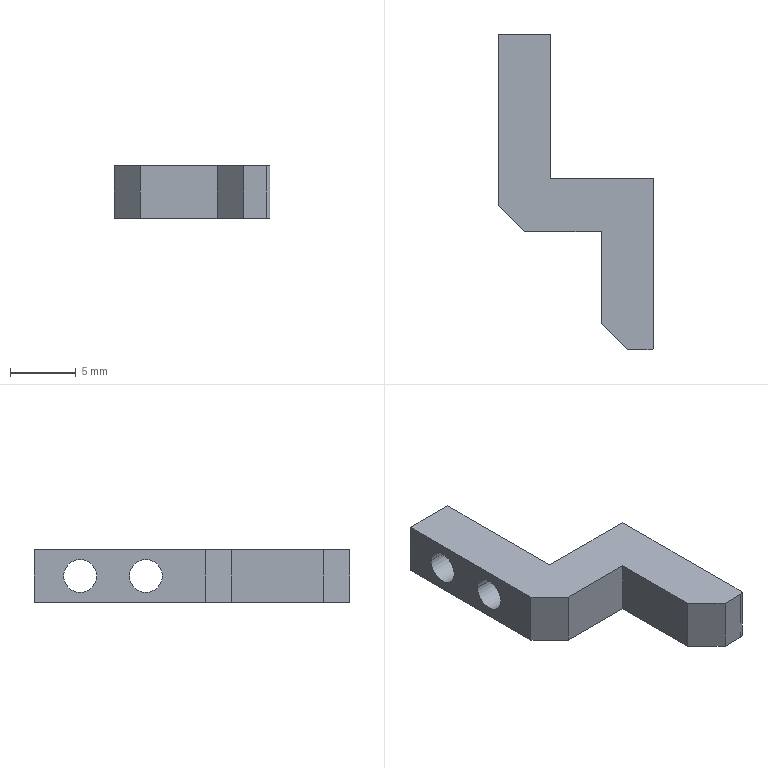Part | STEP file | Gripper_Default | 1 solid | 17 faces | box 11.85 x 24 x 4 mm | volume 454.253 mm3 | plane 12 | cylinder 5 | commonest cylinder face diameters 2.5 x4 0.6 x1
STEP:
#1=CARTESIAN_POINT('',(0.,0.,0.));
#2=DIRECTION('',(0.,0.,1.));
#3=DIRECTION('',(1.,0.,0.));
#4=AXIS2_PLACEMENT_3D('',#1,#2,#3);
#5=CARTESIAN_POINT('',(0.,-2.25,2.));
#6=VERTEX_POINT('',#5);
#7=CARTESIAN_POINT('',(4.,-2.25,2.));
#8=VERTEX_POINT('',#7);
#9=CARTESIAN_POINT('',(0.,-2.25,2.));
#10=DIRECTION('',(1.,0.,0.));
#11=VECTOR('',#10,1.);
#12=LINE('',#9,#11);
#13=CARTESIAN_POINT('',(0.,-3.5,2.));
#14=DIRECTION('',(1.,0.,0.));
#15=DIRECTION('',(0.,1.,0.));
#16=AXIS2_PLACEMENT_3D('',#13,#14,#15);
#17=CYLINDRICAL_SURFACE('',#16,1.25);
#18=CARTESIAN_POINT('',(6.283,0.));
#19=DIRECTION('',(0.,1.));
#20=VECTOR('',#19,1.);
#21=LINE('',#18,#20);
#22=(GEOMETRIC_REPRESENTATION_CONTEXT(2)PARAMETRIC_REPRESENTATION_CONTEXT()REPRESENTATION_CONTEXT('',''));
#23=DEFINITIONAL_REPRESENTATION('',(#21),#22);
#24=PCURVE('',#17,#23);
#25=CARTESIAN_POINT('',(0.,-3.5,2.));
#26=DIRECTION('',(1.,0.,0.));
#27=DIRECTION('',(0.,1.,0.));
#28=AXIS2_PLACEMENT_3D('',#25,#26,#27);
#29=CYLINDRICAL_SURFACE('',#28,1.25);
#30=CARTESIAN_POINT('',(0.,0.));
#31=DIRECTION('',(0.,1.));
#32=VECTOR('',#31,1.);
#33=LINE('',#30,#32);
#34=(GEOMETRIC_REPRESENTATION_CONTEXT(2)PARAMETRIC_REPRESENTATION_CONTEXT()REPRESENTATION_CONTEXT('',''));
#35=DEFINITIONAL_REPRESENTATION('',(#33),#34);
#36=PCURVE('',#29,#35);
#37=SURFACE_CURVE('',#12,(#24,#36),.PCURVE_S1.);
#38=EDGE_CURVE('',#6,#8,#37,.T.);
#39=ORIENTED_EDGE('',*,*,#38,.T.);
#40=CARTESIAN_POINT('',(4.,-4.75,2.));
#41=VERTEX_POINT('',#40);
#42=CARTESIAN_POINT('',(4.,-3.5,2.));
#43=DIRECTION('',(1.,0.,0.));
#44=DIRECTION('',(0.,1.,0.));
#45=AXIS2_PLACEMENT_3D('',#42,#43,#44);
#46=CIRCLE('',#45,1.25);
#47=CARTESIAN_POINT('',(0.,4.));
#48=DIRECTION('',(1.,0.));
#49=VECTOR('',#48,1.);
#50=LINE('',#47,#49);
#51=(GEOMETRIC_REPRESENTATION_CONTEXT(2)PARAMETRIC_REPRESENTATION_CONTEXT()REPRESENTATION_CONTEXT('',''));
#52=DEFINITIONAL_REPRESENTATION('',(#50),#51);
#53=PCURVE('',#17,#52);
#54=CARTESIAN_POINT('',(4.,0.,4.));
#55=DIRECTION('',(-1.,0.,0.));
#56=DIRECTION('',(0.,-1.,0.));
#57=AXIS2_PLACEMENT_3D('',#54,#55,#56);
#58=PLANE('',#57);
#59=CARTESIAN_POINT('',(2.25,-2.));
#60=CARTESIAN_POINT('',(2.25,0.1651));
#61=CARTESIAN_POINT('',(4.125,-0.9175));
#62=CARTESIAN_POINT('',(6.,-2.));
#63=CARTESIAN_POINT('',(4.125,-3.083));
#64=CARTESIAN_POINT('',(2.25,-4.165));
#65=CARTESIAN_POINT('',(2.25,-2.));
#66=(BOUNDED_CURVE()B_SPLINE_CURVE(2,(#59,#60,#61,#62,#63,#64,#65),.UNSPECIFIED.,.T.,.F.)B_SPLINE_CURVE_WITH_KNOTS((1,2,2,2,2,1),(-2.094,0.,2.094,4.189,6.283,8.378),.UNSPECIFIED.)CURVE()GEOMETRIC_REPRESENTATION_ITEM()RATIONAL_B_SPLINE_CURVE((1.,0.5,1.,0.5,1.,0.5,1.))REPRESENTATION_ITEM(''));
#67=(GEOMETRIC_REPRESENTATION_CONTEXT(2)PARAMETRIC_REPRESENTATION_CONTEXT()REPRESENTATION_CONTEXT('',''));
#68=DEFINITIONAL_REPRESENTATION('',(#66),#67);
#69=PCURVE('',#58,#68);
#70=SURFACE_CURVE('',#46,(#53,#69),.PCURVE_S1.);
#71=EDGE_CURVE('',#41,#8,#70,.T.);
#72=ORIENTED_EDGE('',*,*,#71,.F.);
#73=CARTESIAN_POINT('',(0.,-4.75,2.));
#74=VERTEX_POINT('',#73);
#75=CARTESIAN_POINT('',(0.,-4.75,2.));
#76=DIRECTION('',(1.,0.,0.));
#77=VECTOR('',#76,1.);
#78=LINE('',#75,#77);
#79=CARTESIAN_POINT('',(3.142,0.));
#80=DIRECTION('',(0.,1.));
#81=VECTOR('',#80,1.);
#82=LINE('',#79,#81);
#83=(GEOMETRIC_REPRESENTATION_CONTEXT(2)PARAMETRIC_REPRESENTATION_CONTEXT()REPRESENTATION_CONTEXT('',''));
#84=DEFINITIONAL_REPRESENTATION('',(#82),#83);
#85=PCURVE('',#17,#84);
#86=CARTESIAN_POINT('',(3.142,0.));
#87=DIRECTION('',(0.,1.));
#88=VECTOR('',#87,1.);
#89=LINE('',#86,#88);
#90=(GEOMETRIC_REPRESENTATION_CONTEXT(2)PARAMETRIC_REPRESENTATION_CONTEXT()REPRESENTATION_CONTEXT('',''));
#91=DEFINITIONAL_REPRESENTATION('',(#89),#90);
#92=PCURVE('',#29,#91);
#93=SURFACE_CURVE('',#78,(#85,#92),.PCURVE_S1.);
#94=EDGE_CURVE('',#74,#41,#93,.T.);
#95=ORIENTED_EDGE('',*,*,#94,.F.);
#96=CARTESIAN_POINT('',(0.,-3.5,2.));
#97=DIRECTION('',(1.,0.,0.));
#98=DIRECTION('',(0.,1.,0.));
#99=AXIS2_PLACEMENT_3D('',#96,#97,#98);
#100=CIRCLE('',#99,1.25);
#101=CARTESIAN_POINT('',(0.,0.));
#102=DIRECTION('',(1.,0.));
#103=VECTOR('',#102,1.);
#104=LINE('',#101,#103);
#105=(GEOMETRIC_REPRESENTATION_CONTEXT(2)PARAMETRIC_REPRESENTATION_CONTEXT()REPRESENTATION_CONTEXT('',''));
#106=DEFINITIONAL_REPRESENTATION('',(#104),#105);
#107=PCURVE('',#17,#106);
#108=CARTESIAN_POINT('',(0.,0.,4.));
#109=DIRECTION('',(1.,0.,0.));
#110=DIRECTION('',(0.,1.,0.));
#111=AXIS2_PLACEMENT_3D('',#108,#109,#110);
#112=PLANE('',#111);
#113=CARTESIAN_POINT('',(-3.5,-2.));
#114=DIRECTION('',(1.,0.));
#115=AXIS2_PLACEMENT_2D('',#113,#114);
#116=CIRCLE('',#115,1.25);
#117=(GEOMETRIC_REPRESENTATION_CONTEXT(2)PARAMETRIC_REPRESENTATION_CONTEXT()REPRESENTATION_CONTEXT('',''));
#118=DEFINITIONAL_REPRESENTATION('',(#116),#117);
#119=PCURVE('',#112,#118);
#120=SURFACE_CURVE('',#100,(#107,#119),.PCURVE_S1.);
#121=EDGE_CURVE('',#74,#6,#120,.T.);
#122=ORIENTED_EDGE('',*,*,#121,.T.);
#123=EDGE_LOOP('',(#39,#72,#95,#122));
#124=FACE_BOUND('',#123,.F.);
#125=ADVANCED_FACE('',(#124),#17,.F.);
#126=CARTESIAN_POINT('',(0.,-7.25,2.));
#127=VERTEX_POINT('',#126);
#128=CARTESIAN_POINT('',(4.,-7.25,2.));
#129=VERTEX_POINT('',#128);
#130=CARTESIAN_POINT('',(0.,-7.25,2.));
#131=DIRECTION('',(1.,0.,0.));
#132=VECTOR('',#131,1.);
#133=LINE('',#130,#132);
#134=CARTESIAN_POINT('',(0.,-8.5,2.));
#135=DIRECTION('',(1.,0.,0.));
#136=DIRECTION('',(0.,1.,0.));
#137=AXIS2_PLACEMENT_3D('',#134,#135,#136);
#138=CYLINDRICAL_SURFACE('',#137,1.25);
#139=CARTESIAN_POINT('',(6.283,0.));
#140=DIRECTION('',(0.,1.));
#141=VECTOR('',#140,1.);
#142=LINE('',#139,#141);
#143=(GEOMETRIC_REPRESENTATION_CONTEXT(2)PARAMETRIC_REPRESENTATION_CONTEXT()REPRESENTATION_CONTEXT('',''));
#144=DEFINITIONAL_REPRESENTATION('',(#142),#143);
#145=PCURVE('',#138,#144);
#146=CARTESIAN_POINT('',(0.,-8.5,2.));
#147=DIRECTION('',(1.,0.,0.));
#148=DIRECTION('',(0.,1.,0.));
#149=AXIS2_PLACEMENT_3D('',#146,#147,#148);
#150=CYLINDRICAL_SURFACE('',#149,1.25);
#151=CARTESIAN_POINT('',(0.,0.));
#152=DIRECTION('',(0.,1.));
#153=VECTOR('',#152,1.);
#154=LINE('',#151,#153);
#155=(GEOMETRIC_REPRESENTATION_CONTEXT(2)PARAMETRIC_REPRESENTATION_CONTEXT()REPRESENTATION_CONTEXT('',''));
#156=DEFINITIONAL_REPRESENTATION('',(#154),#155);
#157=PCURVE('',#150,#156);
#158=SURFACE_CURVE('',#133,(#145,#157),.PCURVE_S1.);
#159=EDGE_CURVE('',#127,#129,#158,.T.);
#160=ORIENTED_EDGE('',*,*,#159,.T.);
#161=CARTESIAN_POINT('',(4.,-9.75,2.));
#162=VERTEX_POINT('',#161);
#163=CARTESIAN_POINT('',(4.,-8.5,2.));
#164=DIRECTION('',(1.,0.,0.));
#165=DIRECTION('',(0.,1.,0.));
#166=AXIS2_PLACEMENT_3D('',#163,#164,#165);
#167=CIRCLE('',#166,1.25);
#168=CARTESIAN_POINT('',(0.,4.));
#169=DIRECTION('',(1.,0.));
#170=VECTOR('',#169,1.);
#171=LINE('',#168,#170);
#172=(GEOMETRIC_REPRESENTATION_CONTEXT(2)PARAMETRIC_REPRESENTATION_CONTEXT()REPRESENTATION_CONTEXT('',''));
#173=DEFINITIONAL_REPRESENTATION('',(#171),#172);
#174=PCURVE('',#138,#173);
#175=CARTESIAN_POINT('',(7.25,-2.));
#176=CARTESIAN_POINT('',(7.25,0.1651));
#177=CARTESIAN_POINT('',(9.125,-0.9175));
#178=CARTESIAN_POINT('',(11.,-2.));
#179=CARTESIAN_POINT('',(9.125,-3.083));
#180=CARTESIAN_POINT('',(7.25,-4.165));
#181=CARTESIAN_POINT('',(7.25,-2.));
#182=(BOUNDED_CURVE()B_SPLINE_CURVE(2,(#175,#176,#177,#178,#179,#180,#181),.UNSPECIFIED.,.T.,.F.)B_SPLINE_CURVE_WITH_KNOTS((1,2,2,2,2,1),(-2.094,0.,2.094,4.189,6.283,8.378),.UNSPECIFIED.)CURVE()GEOMETRIC_REPRESENTATION_ITEM()RATIONAL_B_SPLINE_CURVE((1.,0.5,1.,0.5,1.,0.5,1.))REPRESENTATION_ITEM(''));
#183=(GEOMETRIC_REPRESENTATION_CONTEXT(2)PARAMETRIC_REPRESENTATION_CONTEXT()REPRESENTATION_CONTEXT('',''));
#184=DEFINITIONAL_REPRESENTATION('',(#182),#183);
#185=PCURVE('',#58,#184);
#186=SURFACE_CURVE('',#167,(#174,#185),.PCURVE_S1.);
#187=EDGE_CURVE('',#162,#129,#186,.T.);
#188=ORIENTED_EDGE('',*,*,#187,.F.);
#189=CARTESIAN_POINT('',(0.,-9.75,2.));
#190=VERTEX_POINT('',#189);
#191=CARTESIAN_POINT('',(0.,-9.75,2.));
#192=DIRECTION('',(1.,0.,0.));
#193=VECTOR('',#192,1.);
#194=LINE('',#191,#193);
#195=CARTESIAN_POINT('',(3.142,0.));
#196=DIRECTION('',(0.,1.));
#197=VECTOR('',#196,1.);
#198=LINE('',#195,#197);
#199=(GEOMETRIC_REPRESENTATION_CONTEXT(2)PARAMETRIC_REPRESENTATION_CONTEXT()REPRESENTATION_CONTEXT('',''));
#200=DEFINITIONAL_REPRESENTATION('',(#198),#199);
#201=PCURVE('',#138,#200);
#202=CARTESIAN_POINT('',(3.142,0.));
#203=DIRECTION('',(0.,1.));
#204=VECTOR('',#203,1.);
#205=LINE('',#202,#204);
#206=(GEOMETRIC_REPRESENTATION_CONTEXT(2)PARAMETRIC_REPRESENTATION_CONTEXT()REPRESENTATION_CONTEXT('',''));
#207=DEFINITIONAL_REPRESENTATION('',(#205),#206);
#208=PCURVE('',#150,#207);
#209=SURFACE_CURVE('',#194,(#201,#208),.PCURVE_S1.);
#210=EDGE_CURVE('',#190,#162,#209,.T.);
#211=ORIENTED_EDGE('',*,*,#210,.F.);
#212=CARTESIAN_POINT('',(0.,-8.5,2.));
#213=DIRECTION('',(1.,0.,0.));
#214=DIRECTION('',(0.,1.,0.));
#215=AXIS2_PLACEMENT_3D('',#212,#213,#214);
#216=CIRCLE('',#215,1.25);
#217=CARTESIAN_POINT('',(0.,0.));
#218=DIRECTION('',(1.,0.));
#219=VECTOR('',#218,1.);
#220=LINE('',#217,#219);
#221=(GEOMETRIC_REPRESENTATION_CONTEXT(2)PARAMETRIC_REPRESENTATION_CONTEXT()REPRESENTATION_CONTEXT('',''));
#222=DEFINITIONAL_REPRESENTATION('',(#220),#221);
#223=PCURVE('',#138,#222);
#224=CARTESIAN_POINT('',(-8.5,-2.));
#225=DIRECTION('',(1.,0.));
#226=AXIS2_PLACEMENT_2D('',#224,#225);
#227=CIRCLE('',#226,1.25);
#228=(GEOMETRIC_REPRESENTATION_CONTEXT(2)PARAMETRIC_REPRESENTATION_CONTEXT()REPRESENTATION_CONTEXT('',''));
#229=DEFINITIONAL_REPRESENTATION('',(#227),#228);
#230=PCURVE('',#112,#229);
#231=SURFACE_CURVE('',#216,(#223,#230),.PCURVE_S1.);
#232=EDGE_CURVE('',#190,#127,#231,.T.);
#233=ORIENTED_EDGE('',*,*,#232,.T.);
#234=EDGE_LOOP('',(#160,#188,#211,#233));
#235=FACE_BOUND('',#234,.F.);
#236=ADVANCED_FACE('',(#235),#138,.F.);
#237=CARTESIAN_POINT('',(0.,-3.5,2.));
#238=DIRECTION('',(1.,0.,0.));
#239=DIRECTION('',(0.,1.,0.));
#240=AXIS2_PLACEMENT_3D('',#237,#238,#239);
#241=CIRCLE('',#240,1.25);
#242=CARTESIAN_POINT('',(-3.5,-2.));
#243=DIRECTION('',(1.,0.));
#244=AXIS2_PLACEMENT_2D('',#242,#243);
#245=CIRCLE('',#244,1.25);
#246=(GEOMETRIC_REPRESENTATION_CONTEXT(2)PARAMETRIC_REPRESENTATION_CONTEXT()REPRESENTATION_CONTEXT('',''));
#247=DEFINITIONAL_REPRESENTATION('',(#245),#246);
#248=PCURVE('',#112,#247);
#249=CARTESIAN_POINT('',(0.,0.));
#250=DIRECTION('',(1.,0.));
#251=VECTOR('',#250,1.);
#252=LINE('',#249,#251);
#253=(GEOMETRIC_REPRESENTATION_CONTEXT(2)PARAMETRIC_REPRESENTATION_CONTEXT()REPRESENTATION_CONTEXT('',''));
#254=DEFINITIONAL_REPRESENTATION('',(#252),#253);
#255=PCURVE('',#29,#254);
#256=SURFACE_CURVE('',#241,(#248,#255),.PCURVE_S1.);
#257=EDGE_CURVE('',#6,#74,#256,.T.);
#258=ORIENTED_EDGE('',*,*,#257,.T.);
#259=ORIENTED_EDGE('',*,*,#121,.T.);
#260=EDGE_LOOP('',(#258,#259));
#261=FACE_BOUND('',#260,.T.);
#262=CARTESIAN_POINT('',(0.,-8.5,2.));
#263=DIRECTION('',(1.,0.,0.));
#264=DIRECTION('',(0.,1.,0.));
#265=AXIS2_PLACEMENT_3D('',#262,#263,#264);
#266=CIRCLE('',#265,1.25);
#267=CARTESIAN_POINT('',(-8.5,-2.));
#268=DIRECTION('',(1.,0.));
#269=AXIS2_PLACEMENT_2D('',#267,#268);
#270=CIRCLE('',#269,1.25);
#271=(GEOMETRIC_REPRESENTATION_CONTEXT(2)PARAMETRIC_REPRESENTATION_CONTEXT()REPRESENTATION_CONTEXT('',''));
#272=DEFINITIONAL_REPRESENTATION('',(#270),#271);
#273=PCURVE('',#112,#272);
#274=CARTESIAN_POINT('',(0.,0.));
#275=DIRECTION('',(1.,0.));
#276=VECTOR('',#275,1.);
#277=LINE('',#274,#276);
#278=(GEOMETRIC_REPRESENTATION_CONTEXT(2)PARAMETRIC_REPRESENTATION_CONTEXT()REPRESENTATION_CONTEXT('',''));
#279=DEFINITIONAL_REPRESENTATION('',(#277),#278);
#280=PCURVE('',#150,#279);
#281=SURFACE_CURVE('',#266,(#273,#280),.PCURVE_S1.);
#282=EDGE_CURVE('',#127,#190,#281,.T.);
#283=ORIENTED_EDGE('',*,*,#282,.T.);
#284=ORIENTED_EDGE('',*,*,#232,.T.);
#285=EDGE_LOOP('',(#283,#284));
#286=FACE_BOUND('',#285,.T.);
#287=CARTESIAN_POINT('',(0.,0.,0.));
#288=VERTEX_POINT('',#287);
#289=CARTESIAN_POINT('',(0.,-13.,0.));
#290=VERTEX_POINT('',#289);
#291=CARTESIAN_POINT('',(0.,0.,0.));
#292=DIRECTION('',(0.,-1.,0.));
#293=VECTOR('',#292,1.);
#294=LINE('',#291,#293);
#295=CARTESIAN_POINT('',(0.,-4.));
#296=DIRECTION('',(-1.,0.));
#297=VECTOR('',#296,1.);
#298=LINE('',#295,#297);
#299=(GEOMETRIC_REPRESENTATION_CONTEXT(2)PARAMETRIC_REPRESENTATION_CONTEXT()REPRESENTATION_CONTEXT('',''));
#300=DEFINITIONAL_REPRESENTATION('',(#298),#299);
#301=PCURVE('',#112,#300);
#302=CARTESIAN_POINT('',(0.,-24.,0.));
#303=DIRECTION('',(0.,0.,-1.));
#304=DIRECTION('',(-1.,0.,0.));
#305=AXIS2_PLACEMENT_3D('',#302,#303,#304);
#306=PLANE('',#305);
#307=CARTESIAN_POINT('',(0.,24.));
#308=DIRECTION('',(0.,-1.));
#309=VECTOR('',#308,1.);
#310=LINE('',#307,#309);
#311=(GEOMETRIC_REPRESENTATION_CONTEXT(2)PARAMETRIC_REPRESENTATION_CONTEXT()REPRESENTATION_CONTEXT('',''));
#312=DEFINITIONAL_REPRESENTATION('',(#310),#311);
#313=PCURVE('',#306,#312);
#314=SURFACE_CURVE('',#294,(#301,#313),.PCURVE_S1.);
#315=EDGE_CURVE('',#288,#290,#314,.T.);
#316=ORIENTED_EDGE('',*,*,#315,.T.);
#317=CARTESIAN_POINT('',(0.,-13.,4.));
#318=VERTEX_POINT('',#317);
#319=CARTESIAN_POINT('',(0.,-13.,4.));
#320=DIRECTION('',(0.,0.,1.));
#321=VECTOR('',#320,1.);
#322=LINE('',#319,#321);
#323=CARTESIAN_POINT('',(-13.,0.));
#324=DIRECTION('',(0.,1.));
#325=VECTOR('',#324,1.);
#326=LINE('',#323,#325);
#327=(GEOMETRIC_REPRESENTATION_CONTEXT(2)PARAMETRIC_REPRESENTATION_CONTEXT()REPRESENTATION_CONTEXT('',''));
#328=DEFINITIONAL_REPRESENTATION('',(#326),#327);
#329=PCURVE('',#112,#328);
#330=CARTESIAN_POINT('',(0.,-13.,4.));
#331=DIRECTION('',(0.7071,0.7071,0.));
#332=DIRECTION('',(-0.7071,0.7071,0.));
#333=AXIS2_PLACEMENT_3D('',#330,#331,#332);
#334=PLANE('',#333);
#335=CARTESIAN_POINT('',(0.,0.));
#336=DIRECTION('',(0.,1.));
#337=VECTOR('',#336,1.);
#338=LINE('',#335,#337);
#339=(GEOMETRIC_REPRESENTATION_CONTEXT(2)PARAMETRIC_REPRESENTATION_CONTEXT()REPRESENTATION_CONTEXT('',''));
#340=DEFINITIONAL_REPRESENTATION('',(#338),#339);
#341=PCURVE('',#334,#340);
#342=SURFACE_CURVE('',#322,(#329,#341),.PCURVE_S1.);
#343=EDGE_CURVE('',#290,#318,#342,.T.);
#344=ORIENTED_EDGE('',*,*,#343,.T.);
#345=CARTESIAN_POINT('',(0.,0.,4.));
#346=VERTEX_POINT('',#345);
#347=CARTESIAN_POINT('',(0.,0.,4.));
#348=DIRECTION('',(0.,-1.,0.));
#349=VECTOR('',#348,1.);
#350=LINE('',#347,#349);
#351=CARTESIAN_POINT('',(0.,0.));
#352=DIRECTION('',(-1.,0.));
#353=VECTOR('',#352,1.);
#354=LINE('',#351,#353);
#355=(GEOMETRIC_REPRESENTATION_CONTEXT(2)PARAMETRIC_REPRESENTATION_CONTEXT()REPRESENTATION_CONTEXT('',''));
#356=DEFINITIONAL_REPRESENTATION('',(#354),#355);
#357=PCURVE('',#112,#356);
#358=CARTESIAN_POINT('',(0.,-24.,4.));
#359=DIRECTION('',(0.,0.,-1.));
#360=DIRECTION('',(-1.,0.,0.));
#361=AXIS2_PLACEMENT_3D('',#358,#359,#360);
#362=PLANE('',#361);
#363=CARTESIAN_POINT('',(0.,24.));
#364=DIRECTION('',(0.,-1.));
#365=VECTOR('',#364,1.);
#366=LINE('',#363,#365);
#367=(GEOMETRIC_REPRESENTATION_CONTEXT(2)PARAMETRIC_REPRESENTATION_CONTEXT()REPRESENTATION_CONTEXT('',''));
#368=DEFINITIONAL_REPRESENTATION('',(#366),#367);
#369=PCURVE('',#362,#368);
#370=SURFACE_CURVE('',#350,(#357,#369),.PCURVE_S1.);
#371=EDGE_CURVE('',#346,#318,#370,.T.);
#372=ORIENTED_EDGE('',*,*,#371,.F.);
#373=CARTESIAN_POINT('',(0.,0.,4.));
#374=DIRECTION('',(0.,0.,-1.));
#375=VECTOR('',#374,1.);
#376=LINE('',#373,#375);
#377=CARTESIAN_POINT('',(0.,0.));
#378=DIRECTION('',(0.,-1.));
#379=VECTOR('',#378,1.);
#380=LINE('',#377,#379);
#381=(GEOMETRIC_REPRESENTATION_CONTEXT(2)PARAMETRIC_REPRESENTATION_CONTEXT()REPRESENTATION_CONTEXT('',''));
#382=DEFINITIONAL_REPRESENTATION('',(#380),#381);
#383=PCURVE('',#112,#382);
#384=CARTESIAN_POINT('',(0.,0.,4.));
#385=DIRECTION('',(0.,-1.,0.));
#386=DIRECTION('',(0.,0.,-1.));
#387=AXIS2_PLACEMENT_3D('',#384,#385,#386);
#388=PLANE('',#387);
#389=CARTESIAN_POINT('',(0.,0.));
#390=DIRECTION('',(1.,0.));
#391=VECTOR('',#390,1.);
#392=LINE('',#389,#391);
#393=(GEOMETRIC_REPRESENTATION_CONTEXT(2)PARAMETRIC_REPRESENTATION_CONTEXT()REPRESENTATION_CONTEXT('',''));
#394=DEFINITIONAL_REPRESENTATION('',(#392),#393);
#395=PCURVE('',#388,#394);
#396=SURFACE_CURVE('',#376,(#383,#395),.PCURVE_S1.);
#397=EDGE_CURVE('',#346,#288,#396,.T.);
#398=ORIENTED_EDGE('',*,*,#397,.T.);
#399=EDGE_LOOP('',(#316,#344,#372,#398));
#400=FACE_BOUND('',#399,.T.);
#401=ADVANCED_FACE('',(#261,#286,#400),#112,.F.);
#402=CARTESIAN_POINT('',(9.85,-24.,0.));
#403=VERTEX_POINT('',#402);
#404=CARTESIAN_POINT('',(11.55,-24.,0.));
#405=VERTEX_POINT('',#404);
#406=CARTESIAN_POINT('',(11.85,-24.,0.));
#407=DIRECTION('',(1.,0.,0.));
#408=VECTOR('',#407,1.);
#409=LINE('',#406,#408);
#410=CARTESIAN_POINT('',(11.85,-24.,4.));
#411=DIRECTION('',(0.,1.,0.));
#412=DIRECTION('',(0.,0.,1.));
#413=AXIS2_PLACEMENT_3D('',#410,#411,#412);
#414=PLANE('',#413);
#415=CARTESIAN_POINT('',(-4.,0.));
#416=DIRECTION('',(0.,1.));
#417=VECTOR('',#416,1.);
#418=LINE('',#415,#417);
#419=(GEOMETRIC_REPRESENTATION_CONTEXT(2)PARAMETRIC_REPRESENTATION_CONTEXT()REPRESENTATION_CONTEXT('',''));
#420=DEFINITIONAL_REPRESENTATION('',(#418),#419);
#421=PCURVE('',#414,#420);
#422=CARTESIAN_POINT('',(-11.85,0.));
#423=DIRECTION('',(-1.,0.));
#424=VECTOR('',#423,1.);
#425=LINE('',#422,#424);
#426=(GEOMETRIC_REPRESENTATION_CONTEXT(2)PARAMETRIC_REPRESENTATION_CONTEXT()REPRESENTATION_CONTEXT('',''));
#427=DEFINITIONAL_REPRESENTATION('',(#425),#426);
#428=PCURVE('',#306,#427);
#429=SURFACE_CURVE('',#409,(#421,#428),.PCURVE_S1.);
#430=EDGE_CURVE('',#403,#405,#429,.T.);
#431=ORIENTED_EDGE('',*,*,#430,.T.);
#432=CARTESIAN_POINT('',(11.55,-24.,4.));
#433=VERTEX_POINT('',#432);
#434=CARTESIAN_POINT('',(11.55,-24.,4.));
#435=DIRECTION('',(0.,0.,1.));
#436=VECTOR('',#435,1.);
#437=LINE('',#434,#436);
#438=CARTESIAN_POINT('',(0.,-0.3));
#439=DIRECTION('',(1.,0.));
#440=VECTOR('',#439,1.);
#441=LINE('',#438,#440);
#442=(GEOMETRIC_REPRESENTATION_CONTEXT(2)PARAMETRIC_REPRESENTATION_CONTEXT()REPRESENTATION_CONTEXT('',''));
#443=DEFINITIONAL_REPRESENTATION('',(#441),#442);
#444=PCURVE('',#414,#443);
#445=CARTESIAN_POINT('',(11.55,-23.7,4.));
#446=DIRECTION('',(0.,0.,-1.));
#447=DIRECTION('',(-1.,0.,0.));
#448=AXIS2_PLACEMENT_3D('',#445,#446,#447);
#449=CYLINDRICAL_SURFACE('',#448,0.3);
#450=CARTESIAN_POINT('',(4.712,0.));
#451=DIRECTION('',(0.,-1.));
#452=VECTOR('',#451,1.);
#453=LINE('',#450,#452);
#454=(GEOMETRIC_REPRESENTATION_CONTEXT(2)PARAMETRIC_REPRESENTATION_CONTEXT()REPRESENTATION_CONTEXT('',''));
#455=DEFINITIONAL_REPRESENTATION('',(#453),#454);
#456=PCURVE('',#449,#455);
#457=SURFACE_CURVE('',#437,(#444,#456),.PCURVE_S1.);
#458=EDGE_CURVE('',#405,#433,#457,.T.);
#459=ORIENTED_EDGE('',*,*,#458,.T.);
#460=CARTESIAN_POINT('',(9.85,-24.,4.));
#461=VERTEX_POINT('',#460);
#462=CARTESIAN_POINT('',(11.85,-24.,4.));
#463=DIRECTION('',(1.,0.,0.));
#464=VECTOR('',#463,1.);
#465=LINE('',#462,#464);
#466=CARTESIAN_POINT('',(0.,0.));
#467=DIRECTION('',(0.,1.));
#468=VECTOR('',#467,1.);
#469=LINE('',#466,#468);
#470=(GEOMETRIC_REPRESENTATION_CONTEXT(2)PARAMETRIC_REPRESENTATION_CONTEXT()REPRESENTATION_CONTEXT('',''));
#471=DEFINITIONAL_REPRESENTATION('',(#469),#470);
#472=PCURVE('',#414,#471);
#473=CARTESIAN_POINT('',(-11.85,0.));
#474=DIRECTION('',(-1.,0.));
#475=VECTOR('',#474,1.);
#476=LINE('',#473,#475);
#477=(GEOMETRIC_REPRESENTATION_CONTEXT(2)PARAMETRIC_REPRESENTATION_CONTEXT()REPRESENTATION_CONTEXT('',''));
#478=DEFINITIONAL_REPRESENTATION('',(#476),#477);
#479=PCURVE('',#362,#478);
#480=SURFACE_CURVE('',#465,(#472,#479),.PCURVE_S1.);
#481=EDGE_CURVE('',#461,#433,#480,.T.);
#482=ORIENTED_EDGE('',*,*,#481,.F.);
#483=CARTESIAN_POINT('',(9.85,-24.,4.));
#484=DIRECTION('',(0.,0.,-1.));
#485=VECTOR('',#484,1.);
#486=LINE('',#483,#485);
#487=CARTESIAN_POINT('',(0.,-2.));
#488=DIRECTION('',(-1.,0.));
#489=VECTOR('',#488,1.);
#490=LINE('',#487,#489);
#491=(GEOMETRIC_REPRESENTATION_CONTEXT(2)PARAMETRIC_REPRESENTATION_CONTEXT()REPRESENTATION_CONTEXT('',''));
#492=DEFINITIONAL_REPRESENTATION('',(#490),#491);
#493=PCURVE('',#414,#492);
#494=CARTESIAN_POINT('',(9.85,-24.,4.));
#495=DIRECTION('',(0.7071,0.7071,0.));
#496=DIRECTION('',(-0.7071,0.7071,0.));
#497=AXIS2_PLACEMENT_3D('',#494,#495,#496);
#498=PLANE('',#497);
#499=CARTESIAN_POINT('',(0.,0.));
#500=DIRECTION('',(0.,-1.));
#501=VECTOR('',#500,1.);
#502=LINE('',#499,#501);
#503=(GEOMETRIC_REPRESENTATION_CONTEXT(2)PARAMETRIC_REPRESENTATION_CONTEXT()REPRESENTATION_CONTEXT('',''));
#504=DEFINITIONAL_REPRESENTATION('',(#502),#503);
#505=PCURVE('',#498,#504);
#506=SURFACE_CURVE('',#486,(#493,#505),.PCURVE_S1.);
#507=EDGE_CURVE('',#461,#403,#506,.T.);
#508=ORIENTED_EDGE('',*,*,#507,.T.);
#509=EDGE_LOOP('',(#431,#459,#482,#508));
#510=FACE_BOUND('',#509,.T.);
#511=ADVANCED_FACE('',(#510),#414,.F.);
#512=CARTESIAN_POINT('',(11.85,-23.7,4.));
#513=VERTEX_POINT('',#512);
#514=CARTESIAN_POINT('',(11.85,-11.,4.));
#515=VERTEX_POINT('',#514);
#516=CARTESIAN_POINT('',(11.85,-11.,4.));
#517=DIRECTION('',(0.,1.,0.));
#518=VECTOR('',#517,1.);
#519=LINE('',#516,#518);
#520=CARTESIAN_POINT('',(11.85,-11.,4.));
#521=DIRECTION('',(-1.,0.,0.));
#522=DIRECTION('',(0.,-1.,0.));
#523=AXIS2_PLACEMENT_3D('',#520,#521,#522);
#524=PLANE('',#523);
#525=CARTESIAN_POINT('',(0.,0.));
#526=DIRECTION('',(-1.,0.));
#527=VECTOR('',#526,1.);
#528=LINE('',#525,#527);
#529=(GEOMETRIC_REPRESENTATION_CONTEXT(2)PARAMETRIC_REPRESENTATION_CONTEXT()REPRESENTATION_CONTEXT('',''));
#530=DEFINITIONAL_REPRESENTATION('',(#528),#529);
#531=PCURVE('',#524,#530);
#532=CARTESIAN_POINT('',(-11.85,13.));
#533=DIRECTION('',(0.,1.));
#534=VECTOR('',#533,1.);
#535=LINE('',#532,#534);
#536=(GEOMETRIC_REPRESENTATION_CONTEXT(2)PARAMETRIC_REPRESENTATION_CONTEXT()REPRESENTATION_CONTEXT('',''));
#537=DEFINITIONAL_REPRESENTATION('',(#535),#536);
#538=PCURVE('',#362,#537);
#539=SURFACE_CURVE('',#519,(#531,#538),.PCURVE_S1.);
#540=EDGE_CURVE('',#513,#515,#539,.T.);
#541=ORIENTED_EDGE('',*,*,#540,.F.);
#542=CARTESIAN_POINT('',(11.85,-23.7,0.));
#543=VERTEX_POINT('',#542);
#544=CARTESIAN_POINT('',(11.85,-23.7,4.));
#545=DIRECTION('',(0.,0.,-1.));
#546=VECTOR('',#545,1.);
#547=LINE('',#544,#546);
#548=CARTESIAN_POINT('',(12.7,0.));
#549=DIRECTION('',(0.,-1.));
#550=VECTOR('',#549,1.);
#551=LINE('',#548,#550);
#552=(GEOMETRIC_REPRESENTATION_CONTEXT(2)PARAMETRIC_REPRESENTATION_CONTEXT()REPRESENTATION_CONTEXT('',''));
#553=DEFINITIONAL_REPRESENTATION('',(#551),#552);
#554=PCURVE('',#524,#553);
#555=CARTESIAN_POINT('',(3.142,0.));
#556=DIRECTION('',(0.,1.));
#557=VECTOR('',#556,1.);
#558=LINE('',#555,#557);
#559=(GEOMETRIC_REPRESENTATION_CONTEXT(2)PARAMETRIC_REPRESENTATION_CONTEXT()REPRESENTATION_CONTEXT('',''));
#560=DEFINITIONAL_REPRESENTATION('',(#558),#559);
#561=PCURVE('',#449,#560);
#562=SURFACE_CURVE('',#547,(#554,#561),.PCURVE_S1.);
#563=EDGE_CURVE('',#513,#543,#562,.T.);
#564=ORIENTED_EDGE('',*,*,#563,.T.);
#565=CARTESIAN_POINT('',(11.85,-11.,0.));
#566=VERTEX_POINT('',#565);
#567=CARTESIAN_POINT('',(11.85,-11.,0.));
#568=DIRECTION('',(0.,1.,0.));
#569=VECTOR('',#568,1.);
#570=LINE('',#567,#569);
#571=CARTESIAN_POINT('',(0.,-4.));
#572=DIRECTION('',(-1.,0.));
#573=VECTOR('',#572,1.);
#574=LINE('',#571,#573);
#575=(GEOMETRIC_REPRESENTATION_CONTEXT(2)PARAMETRIC_REPRESENTATION_CONTEXT()REPRESENTATION_CONTEXT('',''));
#576=DEFINITIONAL_REPRESENTATION('',(#574),#575);
#577=PCURVE('',#524,#576);
#578=CARTESIAN_POINT('',(-11.85,13.));
#579=DIRECTION('',(0.,1.));
#580=VECTOR('',#579,1.);
#581=LINE('',#578,#580);
#582=(GEOMETRIC_REPRESENTATION_CONTEXT(2)PARAMETRIC_REPRESENTATION_CONTEXT()REPRESENTATION_CONTEXT('',''));
#583=DEFINITIONAL_REPRESENTATION('',(#581),#582);
#584=PCURVE('',#306,#583);
#585=SURFACE_CURVE('',#570,(#577,#584),.PCURVE_S1.);
#586=EDGE_CURVE('',#543,#566,#585,.T.);
#587=ORIENTED_EDGE('',*,*,#586,.T.);
#588=CARTESIAN_POINT('',(11.85,-11.,4.));
#589=DIRECTION('',(0.,0.,-1.));
#590=VECTOR('',#589,1.);
#591=LINE('',#588,#590);
#592=CARTESIAN_POINT('',(0.,0.));
#593=DIRECTION('',(0.,-1.));
#594=VECTOR('',#593,1.);
#595=LINE('',#592,#594);
#596=(GEOMETRIC_REPRESENTATION_CONTEXT(2)PARAMETRIC_REPRESENTATION_CONTEXT()REPRESENTATION_CONTEXT('',''));
#597=DEFINITIONAL_REPRESENTATION('',(#595),#596);
#598=PCURVE('',#524,#597);
#599=CARTESIAN_POINT('',(4.,-11.,4.));
#600=DIRECTION('',(0.,-1.,0.));
#601=DIRECTION('',(0.,0.,-1.));
#602=AXIS2_PLACEMENT_3D('',#599,#600,#601);
#603=PLANE('',#602);
#604=CARTESIAN_POINT('',(0.,7.85));
#605=DIRECTION('',(1.,0.));
#606=VECTOR('',#605,1.);
#607=LINE('',#604,#606);
#608=(GEOMETRIC_REPRESENTATION_CONTEXT(2)PARAMETRIC_REPRESENTATION_CONTEXT()REPRESENTATION_CONTEXT('',''));
#609=DEFINITIONAL_REPRESENTATION('',(#607),#608);
#610=PCURVE('',#603,#609);
#611=SURFACE_CURVE('',#591,(#598,#610),.PCURVE_S1.);
#612=EDGE_CURVE('',#515,#566,#611,.T.);
#613=ORIENTED_EDGE('',*,*,#612,.F.);
#614=EDGE_LOOP('',(#541,#564,#587,#613));
#615=FACE_BOUND('',#614,.T.);
#616=ADVANCED_FACE('',(#615),#524,.F.);
#617=CARTESIAN_POINT('',(4.,-11.,0.));
#618=VERTEX_POINT('',#617);
#619=CARTESIAN_POINT('',(4.,-11.,0.));
#620=DIRECTION('',(-1.,0.,0.));
#621=VECTOR('',#620,1.);
#622=LINE('',#619,#621);
#623=CARTESIAN_POINT('',(4.,0.));
#624=DIRECTION('',(0.,-1.));
#625=VECTOR('',#624,1.);
#626=LINE('',#623,#625);
#627=(GEOMETRIC_REPRESENTATION_CONTEXT(2)PARAMETRIC_REPRESENTATION_CONTEXT()REPRESENTATION_CONTEXT('',''));
#628=DEFINITIONAL_REPRESENTATION('',(#626),#627);
#629=PCURVE('',#603,#628);
#630=CARTESIAN_POINT('',(-4.,13.));
#631=DIRECTION('',(1.,0.));
#632=VECTOR('',#631,1.);
#633=LINE('',#630,#632);
#634=(GEOMETRIC_REPRESENTATION_CONTEXT(2)PARAMETRIC_REPRESENTATION_CONTEXT()REPRESENTATION_CONTEXT('',''));
#635=DEFINITIONAL_REPRESENTATION('',(#633),#634);
#636=PCURVE('',#306,#635);
#637=SURFACE_CURVE('',#622,(#629,#636),.PCURVE_S1.);
#638=EDGE_CURVE('',#566,#618,#637,.T.);
#639=ORIENTED_EDGE('',*,*,#638,.T.);
#640=CARTESIAN_POINT('',(4.,-11.,4.));
#641=VERTEX_POINT('',#640);
#642=CARTESIAN_POINT('',(4.,-11.,4.));
#643=DIRECTION('',(0.,0.,-1.));
#644=VECTOR('',#643,1.);
#645=LINE('',#642,#644);
#646=CARTESIAN_POINT('',(0.,0.));
#647=DIRECTION('',(1.,0.));
#648=VECTOR('',#647,1.);
#649=LINE('',#646,#648);
#650=(GEOMETRIC_REPRESENTATION_CONTEXT(2)PARAMETRIC_REPRESENTATION_CONTEXT()REPRESENTATION_CONTEXT('',''));
#651=DEFINITIONAL_REPRESENTATION('',(#649),#650);
#652=PCURVE('',#603,#651);
#653=CARTESIAN_POINT('',(11.,0.));
#654=DIRECTION('',(0.,-1.));
#655=VECTOR('',#654,1.);
#656=LINE('',#653,#655);
#657=(GEOMETRIC_REPRESENTATION_CONTEXT(2)PARAMETRIC_REPRESENTATION_CONTEXT()REPRESENTATION_CONTEXT('',''));
#658=DEFINITIONAL_REPRESENTATION('',(#656),#657);
#659=PCURVE('',#58,#658);
#660=SURFACE_CURVE('',#645,(#652,#659),.PCURVE_S1.);
#661=EDGE_CURVE('',#641,#618,#660,.T.);
#662=ORIENTED_EDGE('',*,*,#661,.F.);
#663=CARTESIAN_POINT('',(4.,-11.,4.));
#664=DIRECTION('',(-1.,0.,0.));
#665=VECTOR('',#664,1.);
#666=LINE('',#663,#665);
#667=CARTESIAN_POINT('',(0.,0.));
#668=DIRECTION('',(0.,-1.));
#669=VECTOR('',#668,1.);
#670=LINE('',#667,#669);
#671=(GEOMETRIC_REPRESENTATION_CONTEXT(2)PARAMETRIC_REPRESENTATION_CONTEXT()REPRESENTATION_CONTEXT('',''));
#672=DEFINITIONAL_REPRESENTATION('',(#670),#671);
#673=PCURVE('',#603,#672);
#674=CARTESIAN_POINT('',(-4.,13.));
#675=DIRECTION('',(1.,0.));
#676=VECTOR('',#675,1.);
#677=LINE('',#674,#676);
#678=(GEOMETRIC_REPRESENTATION_CONTEXT(2)PARAMETRIC_REPRESENTATION_CONTEXT()REPRESENTATION_CONTEXT('',''));
#679=DEFINITIONAL_REPRESENTATION('',(#677),#678);
#680=PCURVE('',#362,#679);
#681=SURFACE_CURVE('',#666,(#673,#680),.PCURVE_S1.);
#682=EDGE_CURVE('',#515,#641,#681,.T.);
#683=ORIENTED_EDGE('',*,*,#682,.F.);
#684=ORIENTED_EDGE('',*,*,#612,.T.);
#685=EDGE_LOOP('',(#639,#662,#683,#684));
#686=FACE_BOUND('',#685,.T.);
#687=ADVANCED_FACE('',(#686),#603,.F.);
#688=CARTESIAN_POINT('',(4.,-3.5,2.));
#689=DIRECTION('',(1.,0.,0.));
#690=DIRECTION('',(0.,1.,0.));
#691=AXIS2_PLACEMENT_3D('',#688,#689,#690);
#692=CIRCLE('',#691,1.25);
#693=CARTESIAN_POINT('',(2.25,-2.));
#694=CARTESIAN_POINT('',(2.25,0.1651));
#695=CARTESIAN_POINT('',(4.125,-0.9175));
#696=CARTESIAN_POINT('',(6.,-2.));
#697=CARTESIAN_POINT('',(4.125,-3.083));
#698=CARTESIAN_POINT('',(2.25,-4.165));
#699=CARTESIAN_POINT('',(2.25,-2.));
#700=(BOUNDED_CURVE()B_SPLINE_CURVE(2,(#693,#694,#695,#696,#697,#698,#699),.UNSPECIFIED.,.T.,.F.)B_SPLINE_CURVE_WITH_KNOTS((1,2,2,2,2,1),(-2.094,0.,2.094,4.189,6.283,8.378),.UNSPECIFIED.)CURVE()GEOMETRIC_REPRESENTATION_ITEM()RATIONAL_B_SPLINE_CURVE((1.,0.5,1.,0.5,1.,0.5,1.))REPRESENTATION_ITEM(''));
#701=(GEOMETRIC_REPRESENTATION_CONTEXT(2)PARAMETRIC_REPRESENTATION_CONTEXT()REPRESENTATION_CONTEXT('',''));
#702=DEFINITIONAL_REPRESENTATION('',(#700),#701);
#703=PCURVE('',#58,#702);
#704=CARTESIAN_POINT('',(0.,4.));
#705=DIRECTION('',(1.,0.));
#706=VECTOR('',#705,1.);
#707=LINE('',#704,#706);
#708=(GEOMETRIC_REPRESENTATION_CONTEXT(2)PARAMETRIC_REPRESENTATION_CONTEXT()REPRESENTATION_CONTEXT('',''));
#709=DEFINITIONAL_REPRESENTATION('',(#707),#708);
#710=PCURVE('',#29,#709);
#711=SURFACE_CURVE('',#692,(#703,#710),.PCURVE_S1.);
#712=EDGE_CURVE('',#8,#41,#711,.T.);
#713=ORIENTED_EDGE('',*,*,#712,.F.);
#714=ORIENTED_EDGE('',*,*,#71,.F.);
#715=EDGE_LOOP('',(#713,#714));
#716=FACE_BOUND('',#715,.T.);
#717=CARTESIAN_POINT('',(4.,-8.5,2.));
#718=DIRECTION('',(1.,0.,0.));
#719=DIRECTION('',(0.,1.,0.));
#720=AXIS2_PLACEMENT_3D('',#717,#718,#719);
#721=CIRCLE('',#720,1.25);
#722=CARTESIAN_POINT('',(7.25,-2.));
#723=CARTESIAN_POINT('',(7.25,0.1651));
#724=CARTESIAN_POINT('',(9.125,-0.9175));
#725=CARTESIAN_POINT('',(11.,-2.));
#726=CARTESIAN_POINT('',(9.125,-3.083));
#727=CARTESIAN_POINT('',(7.25,-4.165));
#728=CARTESIAN_POINT('',(7.25,-2.));
#729=(BOUNDED_CURVE()B_SPLINE_CURVE(2,(#722,#723,#724,#725,#726,#727,#728),.UNSPECIFIED.,.T.,.F.)B_SPLINE_CURVE_WITH_KNOTS((1,2,2,2,2,1),(-2.094,0.,2.094,4.189,6.283,8.378),.UNSPECIFIED.)CURVE()GEOMETRIC_REPRESENTATION_ITEM()RATIONAL_B_SPLINE_CURVE((1.,0.5,1.,0.5,1.,0.5,1.))REPRESENTATION_ITEM(''));
#730=(GEOMETRIC_REPRESENTATION_CONTEXT(2)PARAMETRIC_REPRESENTATION_CONTEXT()REPRESENTATION_CONTEXT('',''));
#731=DEFINITIONAL_REPRESENTATION('',(#729),#730);
#732=PCURVE('',#58,#731);
#733=CARTESIAN_POINT('',(0.,4.));
#734=DIRECTION('',(1.,0.));
#735=VECTOR('',#734,1.);
#736=LINE('',#733,#735);
#737=(GEOMETRIC_REPRESENTATION_CONTEXT(2)PARAMETRIC_REPRESENTATION_CONTEXT()REPRESENTATION_CONTEXT('',''));
#738=DEFINITIONAL_REPRESENTATION('',(#736),#737);
#739=PCURVE('',#150,#738);
#740=SURFACE_CURVE('',#721,(#732,#739),.PCURVE_S1.);
#741=EDGE_CURVE('',#129,#162,#740,.T.);
#742=ORIENTED_EDGE('',*,*,#741,.F.);
#743=ORIENTED_EDGE('',*,*,#187,.F.);
#744=EDGE_LOOP('',(#742,#743));
#745=FACE_BOUND('',#744,.T.);
#746=CARTESIAN_POINT('',(4.,0.,0.));
#747=VERTEX_POINT('',#746);
#748=CARTESIAN_POINT('',(4.,0.,0.));
#749=DIRECTION('',(0.,1.,0.));
#750=VECTOR('',#749,1.);
#751=LINE('',#748,#750);
#752=CARTESIAN_POINT('',(0.,-4.));
#753=DIRECTION('',(-1.,0.));
#754=VECTOR('',#753,1.);
#755=LINE('',#752,#754);
#756=(GEOMETRIC_REPRESENTATION_CONTEXT(2)PARAMETRIC_REPRESENTATION_CONTEXT()REPRESENTATION_CONTEXT('',''));
#757=DEFINITIONAL_REPRESENTATION('',(#755),#756);
#758=PCURVE('',#58,#757);
#759=CARTESIAN_POINT('',(-4.,24.));
#760=DIRECTION('',(0.,1.));
#761=VECTOR('',#760,1.);
#762=LINE('',#759,#761);
#763=(GEOMETRIC_REPRESENTATION_CONTEXT(2)PARAMETRIC_REPRESENTATION_CONTEXT()REPRESENTATION_CONTEXT('',''));
#764=DEFINITIONAL_REPRESENTATION('',(#762),#763);
#765=PCURVE('',#306,#764);
#766=SURFACE_CURVE('',#751,(#758,#765),.PCURVE_S1.);
#767=EDGE_CURVE('',#618,#747,#766,.T.);
#768=ORIENTED_EDGE('',*,*,#767,.T.);
#769=CARTESIAN_POINT('',(4.,0.,4.));
#770=VERTEX_POINT('',#769);
#771=CARTESIAN_POINT('',(4.,0.,4.));
#772=DIRECTION('',(0.,0.,-1.));
#773=VECTOR('',#772,1.);
#774=LINE('',#771,#773);
#775=CARTESIAN_POINT('',(0.,0.));
#776=DIRECTION('',(0.,-1.));
#777=VECTOR('',#776,1.);
#778=LINE('',#775,#777);
#779=(GEOMETRIC_REPRESENTATION_CONTEXT(2)PARAMETRIC_REPRESENTATION_CONTEXT()REPRESENTATION_CONTEXT('',''));
#780=DEFINITIONAL_REPRESENTATION('',(#778),#779);
#781=PCURVE('',#58,#780);
#782=CARTESIAN_POINT('',(0.,4.));
#783=DIRECTION('',(1.,0.));
#784=VECTOR('',#783,1.);
#785=LINE('',#782,#784);
#786=(GEOMETRIC_REPRESENTATION_CONTEXT(2)PARAMETRIC_REPRESENTATION_CONTEXT()REPRESENTATION_CONTEXT('',''));
#787=DEFINITIONAL_REPRESENTATION('',(#785),#786);
#788=PCURVE('',#388,#787);
#789=SURFACE_CURVE('',#774,(#781,#788),.PCURVE_S1.);
#790=EDGE_CURVE('',#770,#747,#789,.T.);
#791=ORIENTED_EDGE('',*,*,#790,.F.);
#792=CARTESIAN_POINT('',(4.,0.,4.));
#793=DIRECTION('',(0.,1.,0.));
#794=VECTOR('',#793,1.);
#795=LINE('',#792,#794);
#796=CARTESIAN_POINT('',(0.,0.));
#797=DIRECTION('',(-1.,0.));
#798=VECTOR('',#797,1.);
#799=LINE('',#796,#798);
#800=(GEOMETRIC_REPRESENTATION_CONTEXT(2)PARAMETRIC_REPRESENTATION_CONTEXT()REPRESENTATION_CONTEXT('',''));
#801=DEFINITIONAL_REPRESENTATION('',(#799),#800);
#802=PCURVE('',#58,#801);
#803=CARTESIAN_POINT('',(-4.,24.));
#804=DIRECTION('',(0.,1.));
#805=VECTOR('',#804,1.);
#806=LINE('',#803,#805);
#807=(GEOMETRIC_REPRESENTATION_CONTEXT(2)PARAMETRIC_REPRESENTATION_CONTEXT()REPRESENTATION_CONTEXT('',''));
#808=DEFINITIONAL_REPRESENTATION('',(#806),#807);
#809=PCURVE('',#362,#808);
#810=SURFACE_CURVE('',#795,(#802,#809),.PCURVE_S1.);
#811=EDGE_CURVE('',#641,#770,#810,.T.);
#812=ORIENTED_EDGE('',*,*,#811,.F.);
#813=ORIENTED_EDGE('',*,*,#661,.T.);
#814=EDGE_LOOP('',(#768,#791,#812,#813));
#815=FACE_BOUND('',#814,.T.);
#816=ADVANCED_FACE('',(#716,#745,#815),#58,.F.);
#817=CARTESIAN_POINT('',(0.,0.,0.));
#818=DIRECTION('',(-1.,0.,0.));
#819=VECTOR('',#818,1.);
#820=LINE('',#817,#819);
#821=CARTESIAN_POINT('',(4.,0.));
#822=DIRECTION('',(0.,-1.));
#823=VECTOR('',#822,1.);
#824=LINE('',#821,#823);
#825=(GEOMETRIC_REPRESENTATION_CONTEXT(2)PARAMETRIC_REPRESENTATION_CONTEXT()REPRESENTATION_CONTEXT('',''));
#826=DEFINITIONAL_REPRESENTATION('',(#824),#825);
#827=PCURVE('',#388,#826);
#828=CARTESIAN_POINT('',(0.,24.));
#829=DIRECTION('',(1.,0.));
#830=VECTOR('',#829,1.);
#831=LINE('',#828,#830);
#832=(GEOMETRIC_REPRESENTATION_CONTEXT(2)PARAMETRIC_REPRESENTATION_CONTEXT()REPRESENTATION_CONTEXT('',''));
#833=DEFINITIONAL_REPRESENTATION('',(#831),#832);
#834=PCURVE('',#306,#833);
#835=SURFACE_CURVE('',#820,(#827,#834),.PCURVE_S1.);
#836=EDGE_CURVE('',#747,#288,#835,.T.);
#837=ORIENTED_EDGE('',*,*,#836,.T.);
#838=ORIENTED_EDGE('',*,*,#397,.F.);
#839=CARTESIAN_POINT('',(0.,0.,4.));
#840=DIRECTION('',(-1.,0.,0.));
#841=VECTOR('',#840,1.);
#842=LINE('',#839,#841);
#843=CARTESIAN_POINT('',(0.,0.));
#844=DIRECTION('',(0.,-1.));
#845=VECTOR('',#844,1.);
#846=LINE('',#843,#845);
#847=(GEOMETRIC_REPRESENTATION_CONTEXT(2)PARAMETRIC_REPRESENTATION_CONTEXT()REPRESENTATION_CONTEXT('',''));
#848=DEFINITIONAL_REPRESENTATION('',(#846),#847);
#849=PCURVE('',#388,#848);
#850=CARTESIAN_POINT('',(0.,24.));
#851=DIRECTION('',(1.,0.));
#852=VECTOR('',#851,1.);
#853=LINE('',#850,#852);
#854=(GEOMETRIC_REPRESENTATION_CONTEXT(2)PARAMETRIC_REPRESENTATION_CONTEXT()REPRESENTATION_CONTEXT('',''));
#855=DEFINITIONAL_REPRESENTATION('',(#853),#854);
#856=PCURVE('',#362,#855);
#857=SURFACE_CURVE('',#842,(#849,#856),.PCURVE_S1.);
#858=EDGE_CURVE('',#770,#346,#857,.T.);
#859=ORIENTED_EDGE('',*,*,#858,.F.);
#860=ORIENTED_EDGE('',*,*,#790,.T.);
#861=EDGE_LOOP('',(#837,#838,#859,#860));
#862=FACE_BOUND('',#861,.T.);
#863=ADVANCED_FACE('',(#862),#388,.F.);
#864=ORIENTED_EDGE('',*,*,#481,.T.);
#865=CARTESIAN_POINT('',(11.55,-23.7,4.));
#866=DIRECTION('',(0.,0.,1.));
#867=DIRECTION('',(-1.,0.,0.));
#868=AXIS2_PLACEMENT_3D('',#865,#866,#867);
#869=CIRCLE('',#868,0.3);
#870=CARTESIAN_POINT('',(-11.25,0.3));
#871=CARTESIAN_POINT('',(-11.25,-0.2196));
#872=CARTESIAN_POINT('',(-11.7,0.04019));
#873=CARTESIAN_POINT('',(-12.15,0.3));
#874=CARTESIAN_POINT('',(-11.7,0.5598));
#875=CARTESIAN_POINT('',(-11.25,0.8196));
#876=CARTESIAN_POINT('',(-11.25,0.3));
#877=(BOUNDED_CURVE()B_SPLINE_CURVE(2,(#870,#871,#872,#873,#874,#875,#876),.UNSPECIFIED.,.T.,.F.)B_SPLINE_CURVE_WITH_KNOTS((1,2,2,2,2,1),(-2.094,0.,2.094,4.189,6.283,8.378),.UNSPECIFIED.)CURVE()GEOMETRIC_REPRESENTATION_ITEM()RATIONAL_B_SPLINE_CURVE((1.,0.5,1.,0.5,1.,0.5,1.))REPRESENTATION_ITEM(''));
#878=(GEOMETRIC_REPRESENTATION_CONTEXT(2)PARAMETRIC_REPRESENTATION_CONTEXT()REPRESENTATION_CONTEXT('',''));
#879=DEFINITIONAL_REPRESENTATION('',(#877),#878);
#880=PCURVE('',#362,#879);
#881=CARTESIAN_POINT('',(6.283,0.));
#882=DIRECTION('',(-1.,0.));
#883=VECTOR('',#882,1.);
#884=LINE('',#881,#883);
#885=(GEOMETRIC_REPRESENTATION_CONTEXT(2)PARAMETRIC_REPRESENTATION_CONTEXT()REPRESENTATION_CONTEXT('',''));
#886=DEFINITIONAL_REPRESENTATION('',(#884),#885);
#887=PCURVE('',#449,#886);
#888=SURFACE_CURVE('',#869,(#880,#887),.PCURVE_S1.);
#889=EDGE_CURVE('',#433,#513,#888,.T.);
#890=ORIENTED_EDGE('',*,*,#889,.T.);
#891=ORIENTED_EDGE('',*,*,#540,.T.);
#892=ORIENTED_EDGE('',*,*,#682,.T.);
#893=ORIENTED_EDGE('',*,*,#811,.T.);
#894=ORIENTED_EDGE('',*,*,#858,.T.);
#895=ORIENTED_EDGE('',*,*,#371,.T.);
#896=CARTESIAN_POINT('',(2.,-15.,4.));
#897=VERTEX_POINT('',#896);
#898=CARTESIAN_POINT('',(0.,-13.,4.));
#899=DIRECTION('',(0.7071,-0.7071,0.));
#900=VECTOR('',#899,1.);
#901=LINE('',#898,#900);
#902=CARTESIAN_POINT('',(0.,11.));
#903=DIRECTION('',(-0.7071,-0.7071));
#904=VECTOR('',#903,1.);
#905=LINE('',#902,#904);
#906=(GEOMETRIC_REPRESENTATION_CONTEXT(2)PARAMETRIC_REPRESENTATION_CONTEXT()REPRESENTATION_CONTEXT('',''));
#907=DEFINITIONAL_REPRESENTATION('',(#905),#906);
#908=PCURVE('',#362,#907);
#909=CARTESIAN_POINT('',(0.,0.));
#910=DIRECTION('',(-1.,0.));
#911=VECTOR('',#910,1.);
#912=LINE('',#909,#911);
#913=(GEOMETRIC_REPRESENTATION_CONTEXT(2)PARAMETRIC_REPRESENTATION_CONTEXT()REPRESENTATION_CONTEXT('',''));
#914=DEFINITIONAL_REPRESENTATION('',(#912),#913);
#915=PCURVE('',#334,#914);
#916=SURFACE_CURVE('',#901,(#908,#915),.PCURVE_S1.);
#917=EDGE_CURVE('',#318,#897,#916,.T.);
#918=ORIENTED_EDGE('',*,*,#917,.T.);
#919=CARTESIAN_POINT('',(7.85,-15.,4.));
#920=VERTEX_POINT('',#919);
#921=CARTESIAN_POINT('',(7.85,-15.,4.));
#922=DIRECTION('',(-1.,0.,0.));
#923=VECTOR('',#922,1.);
#924=LINE('',#921,#923);
#925=CARTESIAN_POINT('',(-7.85,9.));
#926=DIRECTION('',(1.,0.));
#927=VECTOR('',#926,1.);
#928=LINE('',#925,#927);
#929=(GEOMETRIC_REPRESENTATION_CONTEXT(2)PARAMETRIC_REPRESENTATION_CONTEXT()REPRESENTATION_CONTEXT('',''));
#930=DEFINITIONAL_REPRESENTATION('',(#928),#929);
#931=PCURVE('',#362,#930);
#932=CARTESIAN_POINT('',(7.85,-15.,0.));
#933=DIRECTION('',(0.,1.,0.));
#934=DIRECTION('',(-1.,0.,0.));
#935=AXIS2_PLACEMENT_3D('',#932,#933,#934);
#936=PLANE('',#935);
#937=CARTESIAN_POINT('',(0.,4.));
#938=DIRECTION('',(1.,0.));
#939=VECTOR('',#938,1.);
#940=LINE('',#937,#939);
#941=(GEOMETRIC_REPRESENTATION_CONTEXT(2)PARAMETRIC_REPRESENTATION_CONTEXT()REPRESENTATION_CONTEXT('',''));
#942=DEFINITIONAL_REPRESENTATION('',(#940),#941);
#943=PCURVE('',#936,#942);
#944=SURFACE_CURVE('',#924,(#931,#943),.PCURVE_S1.);
#945=EDGE_CURVE('',#920,#897,#944,.T.);
#946=ORIENTED_EDGE('',*,*,#945,.F.);
#947=CARTESIAN_POINT('',(7.85,-22.,4.));
#948=VERTEX_POINT('',#947);
#949=CARTESIAN_POINT('',(7.85,-15.,4.));
#950=DIRECTION('',(0.,1.,0.));
#951=VECTOR('',#950,1.);
#952=LINE('',#949,#951);
#953=CARTESIAN_POINT('',(-7.85,9.));
#954=DIRECTION('',(0.,1.));
#955=VECTOR('',#954,1.);
#956=LINE('',#953,#955);
#957=(GEOMETRIC_REPRESENTATION_CONTEXT(2)PARAMETRIC_REPRESENTATION_CONTEXT()REPRESENTATION_CONTEXT('',''));
#958=DEFINITIONAL_REPRESENTATION('',(#956),#957);
#959=PCURVE('',#362,#958);
#960=CARTESIAN_POINT('',(7.85,-15.,0.));
#961=DIRECTION('',(1.,0.,0.));
#962=DIRECTION('',(0.,1.,0.));
#963=AXIS2_PLACEMENT_3D('',#960,#961,#962);
#964=PLANE('',#963);
#965=CARTESIAN_POINT('',(0.,4.));
#966=DIRECTION('',(1.,0.));
#967=VECTOR('',#966,1.);
#968=LINE('',#965,#967);
#969=(GEOMETRIC_REPRESENTATION_CONTEXT(2)PARAMETRIC_REPRESENTATION_CONTEXT()REPRESENTATION_CONTEXT('',''));
#970=DEFINITIONAL_REPRESENTATION('',(#968),#969);
#971=PCURVE('',#964,#970);
#972=SURFACE_CURVE('',#952,(#959,#971),.PCURVE_S1.);
#973=EDGE_CURVE('',#948,#920,#972,.T.);
#974=ORIENTED_EDGE('',*,*,#973,.F.);
#975=CARTESIAN_POINT('',(9.85,-24.,4.));
#976=DIRECTION('',(0.7071,-0.7071,0.));
#977=VECTOR('',#976,1.);
#978=LINE('',#975,#977);
#979=CARTESIAN_POINT('',(-9.85,0.));
#980=DIRECTION('',(-0.7071,-0.7071));
#981=VECTOR('',#980,1.);
#982=LINE('',#979,#981);
#983=(GEOMETRIC_REPRESENTATION_CONTEXT(2)PARAMETRIC_REPRESENTATION_CONTEXT()REPRESENTATION_CONTEXT('',''));
#984=DEFINITIONAL_REPRESENTATION('',(#982),#983);
#985=PCURVE('',#362,#984);
#986=CARTESIAN_POINT('',(0.,0.));
#987=DIRECTION('',(-1.,0.));
#988=VECTOR('',#987,1.);
#989=LINE('',#986,#988);
#990=(GEOMETRIC_REPRESENTATION_CONTEXT(2)PARAMETRIC_REPRESENTATION_CONTEXT()REPRESENTATION_CONTEXT('',''));
#991=DEFINITIONAL_REPRESENTATION('',(#989),#990);
#992=PCURVE('',#498,#991);
#993=SURFACE_CURVE('',#978,(#985,#992),.PCURVE_S1.);
#994=EDGE_CURVE('',#948,#461,#993,.T.);
#995=ORIENTED_EDGE('',*,*,#994,.T.);
#996=EDGE_LOOP('',(#864,#890,#891,#892,#893,#894,#895,#918,#946,#974,#995));
#997=FACE_BOUND('',#996,.T.);
#998=ADVANCED_FACE('',(#997),#362,.F.);
#999=ORIENTED_EDGE('',*,*,#586,.F.);
#1000=CARTESIAN_POINT('',(11.55,-23.7,0.));
#1001=DIRECTION('',(0.,0.,-1.));
#1002=DIRECTION('',(-1.,0.,0.));
#1003=AXIS2_PLACEMENT_3D('',#1000,#1001,#1002);
#1004=CIRCLE('',#1003,0.3);
#1005=CARTESIAN_POINT('',(-11.55,0.3));
#1006=DIRECTION('',(1.,0.));
#1007=AXIS2_PLACEMENT_2D('',#1005,#1006);
#1008=CIRCLE('',#1007,0.3);
#1009=(GEOMETRIC_REPRESENTATION_CONTEXT(2)PARAMETRIC_REPRESENTATION_CONTEXT()REPRESENTATION_CONTEXT('',''));
#1010=DEFINITIONAL_REPRESENTATION('',(#1008),#1009);
#1011=PCURVE('',#306,#1010);
#1012=CARTESIAN_POINT('',(0.,4.));
#1013=DIRECTION('',(1.,0.));
#1014=VECTOR('',#1013,1.);
#1015=LINE('',#1012,#1014);
#1016=(GEOMETRIC_REPRESENTATION_CONTEXT(2)PARAMETRIC_REPRESENTATION_CONTEXT()REPRESENTATION_CONTEXT('',''));
#1017=DEFINITIONAL_REPRESENTATION('',(#1015),#1016);
#1018=PCURVE('',#449,#1017);
#1019=SURFACE_CURVE('',#1004,(#1011,#1018),.PCURVE_S1.);
#1020=EDGE_CURVE('',#543,#405,#1019,.T.);
#1021=ORIENTED_EDGE('',*,*,#1020,.T.);
#1022=ORIENTED_EDGE('',*,*,#430,.F.);
#1023=CARTESIAN_POINT('',(7.85,-22.,0.));
#1024=VERTEX_POINT('',#1023);
#1025=CARTESIAN_POINT('',(4.925,-19.075,0.));
#1026=DIRECTION('',(-0.7071,0.7071,0.));
#1027=VECTOR('',#1026,1.);
#1028=LINE('',#1025,#1027);
#1029=CARTESIAN_POINT('',(-4.925,4.925));
#1030=DIRECTION('',(0.7071,0.7071));
#1031=VECTOR('',#1030,1.);
#1032=LINE('',#1029,#1031);
#1033=(GEOMETRIC_REPRESENTATION_CONTEXT(2)PARAMETRIC_REPRESENTATION_CONTEXT()REPRESENTATION_CONTEXT('',''));
#1034=DEFINITIONAL_REPRESENTATION('',(#1032),#1033);
#1035=PCURVE('',#306,#1034);
#1036=CARTESIAN_POINT('',(6.965,-4.));
#1037=DIRECTION('',(1.,0.));
#1038=VECTOR('',#1037,1.);
#1039=LINE('',#1036,#1038);
#1040=(GEOMETRIC_REPRESENTATION_CONTEXT(2)PARAMETRIC_REPRESENTATION_CONTEXT()REPRESENTATION_CONTEXT('',''));
#1041=DEFINITIONAL_REPRESENTATION('',(#1039),#1040);
#1042=PCURVE('',#498,#1041);
#1043=SURFACE_CURVE('',#1028,(#1035,#1042),.PCURVE_S1.);
#1044=EDGE_CURVE('',#403,#1024,#1043,.T.);
#1045=ORIENTED_EDGE('',*,*,#1044,.T.);
#1046=CARTESIAN_POINT('',(7.85,-15.,0.));
#1047=VERTEX_POINT('',#1046);
#1048=CARTESIAN_POINT('',(7.85,-24.,0.));
#1049=DIRECTION('',(0.,-1.,0.));
#1050=VECTOR('',#1049,1.);
#1051=LINE('',#1048,#1050);
#1052=CARTESIAN_POINT('',(-7.85,0.));
#1053=DIRECTION('',(0.,-1.));
#1054=VECTOR('',#1053,1.);
#1055=LINE('',#1052,#1054);
#1056=(GEOMETRIC_REPRESENTATION_CONTEXT(2)PARAMETRIC_REPRESENTATION_CONTEXT()REPRESENTATION_CONTEXT('',''));
#1057=DEFINITIONAL_REPRESENTATION('',(#1055),#1056);
#1058=PCURVE('',#306,#1057);
#1059=CARTESIAN_POINT('',(-9.,0.));
#1060=DIRECTION('',(-1.,0.));
#1061=VECTOR('',#1060,1.);
#1062=LINE('',#1059,#1061);
#1063=(GEOMETRIC_REPRESENTATION_CONTEXT(2)PARAMETRIC_REPRESENTATION_CONTEXT()REPRESENTATION_CONTEXT('',''));
#1064=DEFINITIONAL_REPRESENTATION('',(#1062),#1063);
#1065=PCURVE('',#964,#1064);
#1066=SURFACE_CURVE('',#1051,(#1058,#1065),.PCURVE_S1.);
#1067=EDGE_CURVE('',#1047,#1024,#1066,.T.);
#1068=ORIENTED_EDGE('',*,*,#1067,.F.);
#1069=CARTESIAN_POINT('',(2.,-15.,0.));
#1070=VERTEX_POINT('',#1069);
#1071=CARTESIAN_POINT('',(7.85,-15.,0.));
#1072=DIRECTION('',(-1.,0.,0.));
#1073=VECTOR('',#1072,1.);
#1074=LINE('',#1071,#1073);
#1075=CARTESIAN_POINT('',(-7.85,9.));
#1076=DIRECTION('',(1.,0.));
#1077=VECTOR('',#1076,1.);
#1078=LINE('',#1075,#1077);
#1079=(GEOMETRIC_REPRESENTATION_CONTEXT(2)PARAMETRIC_REPRESENTATION_CONTEXT()REPRESENTATION_CONTEXT('',''));
#1080=DEFINITIONAL_REPRESENTATION('',(#1078),#1079);
#1081=PCURVE('',#306,#1080);
#1082=CARTESIAN_POINT('',(0.,0.));
#1083=DIRECTION('',(1.,0.));
#1084=VECTOR('',#1083,1.);
#1085=LINE('',#1082,#1084);
#1086=(GEOMETRIC_REPRESENTATION_CONTEXT(2)PARAMETRIC_REPRESENTATION_CONTEXT()REPRESENTATION_CONTEXT('',''));
#1087=DEFINITIONAL_REPRESENTATION('',(#1085),#1086);
#1088=PCURVE('',#936,#1087);
#1089=SURFACE_CURVE('',#1074,(#1081,#1088),.PCURVE_S1.);
#1090=EDGE_CURVE('',#1047,#1070,#1089,.T.);
#1091=ORIENTED_EDGE('',*,*,#1090,.T.);
#1092=CARTESIAN_POINT('',(5.5,-18.5,0.));
#1093=DIRECTION('',(-0.7071,0.7071,0.));
#1094=VECTOR('',#1093,1.);
#1095=LINE('',#1092,#1094);
#1096=CARTESIAN_POINT('',(-5.5,5.5));
#1097=DIRECTION('',(0.7071,0.7071));
#1098=VECTOR('',#1097,1.);
#1099=LINE('',#1096,#1098);
#1100=(GEOMETRIC_REPRESENTATION_CONTEXT(2)PARAMETRIC_REPRESENTATION_CONTEXT()REPRESENTATION_CONTEXT('',''));
#1101=DEFINITIONAL_REPRESENTATION('',(#1099),#1100);
#1102=PCURVE('',#306,#1101);
#1103=CARTESIAN_POINT('',(-7.778,-4.));
#1104=DIRECTION('',(1.,0.));
#1105=VECTOR('',#1104,1.);
#1106=LINE('',#1103,#1105);
#1107=(GEOMETRIC_REPRESENTATION_CONTEXT(2)PARAMETRIC_REPRESENTATION_CONTEXT()REPRESENTATION_CONTEXT('',''));
#1108=DEFINITIONAL_REPRESENTATION('',(#1106),#1107);
#1109=PCURVE('',#334,#1108);
#1110=SURFACE_CURVE('',#1095,(#1102,#1109),.PCURVE_S1.);
#1111=EDGE_CURVE('',#1070,#290,#1110,.T.);
#1112=ORIENTED_EDGE('',*,*,#1111,.T.);
#1113=ORIENTED_EDGE('',*,*,#315,.F.);
#1114=ORIENTED_EDGE('',*,*,#836,.F.);
#1115=ORIENTED_EDGE('',*,*,#767,.F.);
#1116=ORIENTED_EDGE('',*,*,#638,.F.);
#1117=EDGE_LOOP('',(#999,#1021,#1022,#1045,#1068,#1091,#1112,#1113,#1114,#1115,#1116));
#1118=FACE_BOUND('',#1117,.T.);
#1119=ADVANCED_FACE('',(#1118),#306,.T.);
#1120=ORIENTED_EDGE('',*,*,#741,.F.);
#1121=ORIENTED_EDGE('',*,*,#159,.F.);
#1122=ORIENTED_EDGE('',*,*,#282,.T.);
#1123=ORIENTED_EDGE('',*,*,#210,.T.);
#1124=EDGE_LOOP('',(#1120,#1121,#1122,#1123));
#1125=FACE_BOUND('',#1124,.F.);
#1126=ADVANCED_FACE('',(#1125),#150,.F.);
#1127=ORIENTED_EDGE('',*,*,#712,.F.);
#1128=ORIENTED_EDGE('',*,*,#38,.F.);
#1129=ORIENTED_EDGE('',*,*,#257,.T.);
#1130=ORIENTED_EDGE('',*,*,#94,.T.);
#1131=EDGE_LOOP('',(#1127,#1128,#1129,#1130));
#1132=FACE_BOUND('',#1131,.F.);
#1133=ADVANCED_FACE('',(#1132),#29,.F.);
#1134=ORIENTED_EDGE('',*,*,#1067,.T.);
#1135=CARTESIAN_POINT('',(7.85,-22.,0.));
#1136=DIRECTION('',(0.,0.,1.));
#1137=VECTOR('',#1136,1.);
#1138=LINE('',#1135,#1137);
#1139=CARTESIAN_POINT('',(-7.,0.));
#1140=DIRECTION('',(0.,1.));
#1141=VECTOR('',#1140,1.);
#1142=LINE('',#1139,#1141);
#1143=(GEOMETRIC_REPRESENTATION_CONTEXT(2)PARAMETRIC_REPRESENTATION_CONTEXT()REPRESENTATION_CONTEXT('',''));
#1144=DEFINITIONAL_REPRESENTATION('',(#1142),#1143);
#1145=PCURVE('',#964,#1144);
#1146=CARTESIAN_POINT('',(2.828,-4.));
#1147=DIRECTION('',(0.,1.));
#1148=VECTOR('',#1147,1.);
#1149=LINE('',#1146,#1148);
#1150=(GEOMETRIC_REPRESENTATION_CONTEXT(2)PARAMETRIC_REPRESENTATION_CONTEXT()REPRESENTATION_CONTEXT('',''));
#1151=DEFINITIONAL_REPRESENTATION('',(#1149),#1150);
#1152=PCURVE('',#498,#1151);
#1153=SURFACE_CURVE('',#1138,(#1145,#1152),.PCURVE_S1.);
#1154=EDGE_CURVE('',#1024,#948,#1153,.T.);
#1155=ORIENTED_EDGE('',*,*,#1154,.T.);
#1156=ORIENTED_EDGE('',*,*,#973,.T.);
#1157=CARTESIAN_POINT('',(7.85,-15.,0.));
#1158=DIRECTION('',(0.,0.,1.));
#1159=VECTOR('',#1158,1.);
#1160=LINE('',#1157,#1159);
#1161=CARTESIAN_POINT('',(0.,0.));
#1162=DIRECTION('',(0.,1.));
#1163=VECTOR('',#1162,1.);
#1164=LINE('',#1161,#1163);
#1165=(GEOMETRIC_REPRESENTATION_CONTEXT(2)PARAMETRIC_REPRESENTATION_CONTEXT()REPRESENTATION_CONTEXT('',''));
#1166=DEFINITIONAL_REPRESENTATION('',(#1164),#1165);
#1167=PCURVE('',#964,#1166);
#1168=CARTESIAN_POINT('',(0.,0.));
#1169=DIRECTION('',(0.,1.));
#1170=VECTOR('',#1169,1.);
#1171=LINE('',#1168,#1170);
#1172=(GEOMETRIC_REPRESENTATION_CONTEXT(2)PARAMETRIC_REPRESENTATION_CONTEXT()REPRESENTATION_CONTEXT('',''));
#1173=DEFINITIONAL_REPRESENTATION('',(#1171),#1172);
#1174=PCURVE('',#936,#1173);
#1175=SURFACE_CURVE('',#1160,(#1167,#1174),.PCURVE_S1.);
#1176=EDGE_CURVE('',#1047,#920,#1175,.T.);
#1177=ORIENTED_EDGE('',*,*,#1176,.F.);
#1178=EDGE_LOOP('',(#1134,#1155,#1156,#1177));
#1179=FACE_BOUND('',#1178,.T.);
#1180=ADVANCED_FACE('',(#1179),#964,.F.);
#1181=ORIENTED_EDGE('',*,*,#945,.T.);
#1182=CARTESIAN_POINT('',(2.,-15.,0.));
#1183=DIRECTION('',(0.,0.,-1.));
#1184=VECTOR('',#1183,1.);
#1185=LINE('',#1182,#1184);
#1186=CARTESIAN_POINT('',(5.85,0.));
#1187=DIRECTION('',(0.,-1.));
#1188=VECTOR('',#1187,1.);
#1189=LINE('',#1186,#1188);
#1190=(GEOMETRIC_REPRESENTATION_CONTEXT(2)PARAMETRIC_REPRESENTATION_CONTEXT()REPRESENTATION_CONTEXT('',''));
#1191=DEFINITIONAL_REPRESENTATION('',(#1189),#1190);
#1192=PCURVE('',#936,#1191);
#1193=CARTESIAN_POINT('',(-2.828,-4.));
#1194=DIRECTION('',(0.,-1.));
#1195=VECTOR('',#1194,1.);
#1196=LINE('',#1193,#1195);
#1197=(GEOMETRIC_REPRESENTATION_CONTEXT(2)PARAMETRIC_REPRESENTATION_CONTEXT()REPRESENTATION_CONTEXT('',''));
#1198=DEFINITIONAL_REPRESENTATION('',(#1196),#1197);
#1199=PCURVE('',#334,#1198);
#1200=SURFACE_CURVE('',#1185,(#1192,#1199),.PCURVE_S1.);
#1201=EDGE_CURVE('',#897,#1070,#1200,.T.);
#1202=ORIENTED_EDGE('',*,*,#1201,.T.);
#1203=ORIENTED_EDGE('',*,*,#1090,.F.);
#1204=ORIENTED_EDGE('',*,*,#1176,.T.);
#1205=EDGE_LOOP('',(#1181,#1202,#1203,#1204));
#1206=FACE_BOUND('',#1205,.T.);
#1207=ADVANCED_FACE('',(#1206),#936,.F.);
#1208=ORIENTED_EDGE('',*,*,#1111,.F.);
#1209=ORIENTED_EDGE('',*,*,#1201,.F.);
#1210=ORIENTED_EDGE('',*,*,#917,.F.);
#1211=ORIENTED_EDGE('',*,*,#343,.F.);
#1212=EDGE_LOOP('',(#1208,#1209,#1210,#1211));
#1213=FACE_BOUND('',#1212,.T.);
#1214=ADVANCED_FACE('',(#1213),#334,.F.);
#1215=ORIENTED_EDGE('',*,*,#994,.F.);
#1216=ORIENTED_EDGE('',*,*,#1154,.F.);
#1217=ORIENTED_EDGE('',*,*,#1044,.F.);
#1218=ORIENTED_EDGE('',*,*,#507,.F.);
#1219=EDGE_LOOP('',(#1215,#1216,#1217,#1218));
#1220=FACE_BOUND('',#1219,.T.);
#1221=ADVANCED_FACE('',(#1220),#498,.F.);
#1222=ORIENTED_EDGE('',*,*,#889,.F.);
#1223=ORIENTED_EDGE('',*,*,#458,.F.);
#1224=ORIENTED_EDGE('',*,*,#1020,.F.);
#1225=ORIENTED_EDGE('',*,*,#563,.F.);
#1226=EDGE_LOOP('',(#1222,#1223,#1224,#1225));
#1227=FACE_BOUND('',#1226,.T.);
#1228=ADVANCED_FACE('',(#1227),#449,.T.);
#1229=CLOSED_SHELL('',(#125,#236,#401,#511,#616,#687,#816,#863,#998,#1119,#1126,#1133,#1180,#1207,#1214,#1221,#1228));
#1230=MANIFOLD_SOLID_BREP('',#1229);
#1231=(LENGTH_UNIT()NAMED_UNIT(*)SI_UNIT(.MILLI.,.METRE.));
#1232=UNCERTAINTY_MEASURE_WITH_UNIT(LENGTH_MEASURE(0.0000001),#1231,'','');
#1233=(NAMED_UNIT(*)PLANE_ANGLE_UNIT()SI_UNIT($,.RADIAN.));
#1234=(NAMED_UNIT(*)SI_UNIT($,.STERADIAN.)SOLID_ANGLE_UNIT());
#1235=(GEOMETRIC_REPRESENTATION_CONTEXT(3)GLOBAL_UNCERTAINTY_ASSIGNED_CONTEXT((#1232))GLOBAL_UNIT_ASSIGNED_CONTEXT((#1231,#1233,#1234))REPRESENTATION_CONTEXT('',''));
#1236=ADVANCED_BREP_SHAPE_REPRESENTATION('',(#4,#1230),#1235);